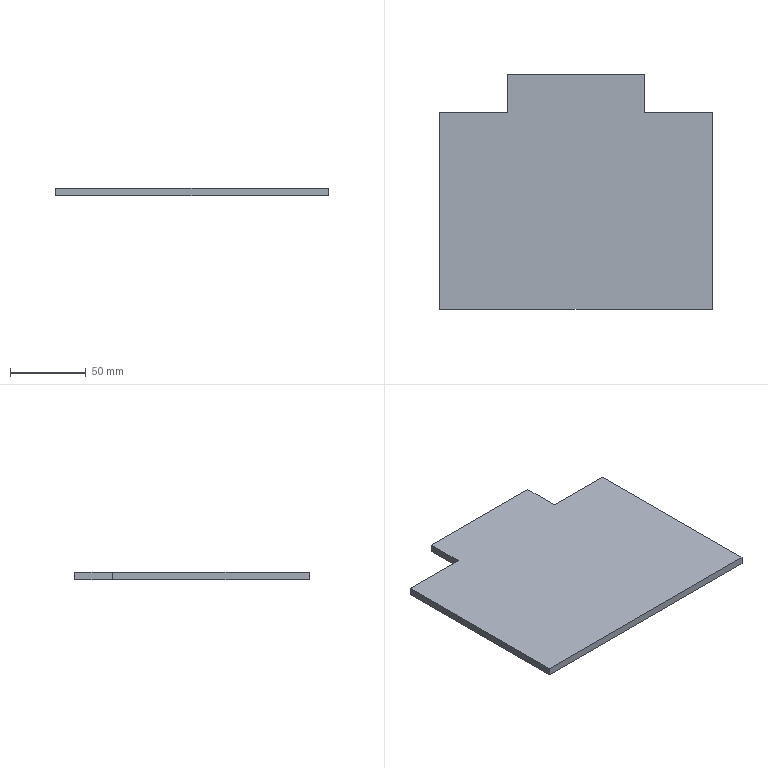Part | SolidWorks | features Extrusion 1, ICE 1 | 1 solid | 10 faces | box 180 x 155 x 5 mm | volume 128250 mm3 | plane 10
STEP:
#1=CARTESIAN_POINT('',(135.,0.,5.));
#2=VERTEX_POINT('',#1);
#3=CARTESIAN_POINT('',(135.,0.,0.));
#4=VERTEX_POINT('',#3);
#5=CARTESIAN_POINT('',(135.,0.,5.));
#6=DIRECTION('',(0.,0.,-1.));
#7=VECTOR('',#6,1000.);
#8=LINE('',#5,#7);
#9=EDGE_CURVE('',#2,#4,#8,.T.);
#10=ORIENTED_EDGE('',*,*,#9,.F.);
#11=CARTESIAN_POINT('',(180.,0.,5.));
#12=VERTEX_POINT('',#11);
#13=CARTESIAN_POINT('',(0.,0.,5.));
#14=DIRECTION('',(-1.,0.,0.));
#15=VECTOR('',#14,1000.);
#16=LINE('',#13,#15);
#17=EDGE_CURVE('',#12,#2,#16,.T.);
#18=ORIENTED_EDGE('',*,*,#17,.F.);
#19=CARTESIAN_POINT('',(180.,0.,0.));
#20=VERTEX_POINT('',#19);
#21=CARTESIAN_POINT('',(180.,0.,5.));
#22=DIRECTION('',(0.,0.,-1.));
#23=VECTOR('',#22,1000.);
#24=LINE('',#21,#23);
#25=EDGE_CURVE('',#12,#20,#24,.T.);
#26=ORIENTED_EDGE('',*,*,#25,.T.);
#27=CARTESIAN_POINT('',(0.,0.,0.));
#28=DIRECTION('',(-1.,0.,0.));
#29=VECTOR('',#28,1000.);
#30=LINE('',#27,#29);
#31=EDGE_CURVE('',#20,#4,#30,.T.);
#32=ORIENTED_EDGE('',*,*,#31,.T.);
#33=EDGE_LOOP('',(#10,#18,#26,#32));
#34=FACE_OUTER_BOUND('',#33,.T.);
#35=CARTESIAN_POINT('',(0.,0.,5.));
#36=DIRECTION('',(0.,-1.,0.));
#37=DIRECTION('',(0.,0.,-1.));
#38=AXIS2_PLACEMENT_3D('',#35,#36,#37);
#39=PLANE('',#38);
#40=ADVANCED_FACE('',(#34),#39,.F.);
#41=CARTESIAN_POINT('',(45.,0.,0.));
#42=VERTEX_POINT('',#41);
#43=CARTESIAN_POINT('',(45.,0.,5.));
#44=VERTEX_POINT('',#43);
#45=CARTESIAN_POINT('',(45.,0.,0.));
#46=DIRECTION('',(0.,0.,1.));
#47=VECTOR('',#46,1000.);
#48=LINE('',#45,#47);
#49=EDGE_CURVE('',#42,#44,#48,.T.);
#50=ORIENTED_EDGE('',*,*,#49,.F.);
#51=CARTESIAN_POINT('',(0.,0.,0.));
#52=VERTEX_POINT('',#51);
#53=CARTESIAN_POINT('',(0.,0.,0.));
#54=DIRECTION('',(-1.,0.,0.));
#55=VECTOR('',#54,1000.);
#56=LINE('',#53,#55);
#57=EDGE_CURVE('',#42,#52,#56,.T.);
#58=ORIENTED_EDGE('',*,*,#57,.T.);
#59=CARTESIAN_POINT('',(0.,0.,5.));
#60=VERTEX_POINT('',#59);
#61=CARTESIAN_POINT('',(0.,0.,5.));
#62=DIRECTION('',(0.,0.,-1.));
#63=VECTOR('',#62,1000.);
#64=LINE('',#61,#63);
#65=EDGE_CURVE('',#60,#52,#64,.T.);
#66=ORIENTED_EDGE('',*,*,#65,.F.);
#67=CARTESIAN_POINT('',(0.,0.,5.));
#68=DIRECTION('',(-1.,0.,0.));
#69=VECTOR('',#68,1000.);
#70=LINE('',#67,#69);
#71=EDGE_CURVE('',#44,#60,#70,.T.);
#72=ORIENTED_EDGE('',*,*,#71,.F.);
#73=EDGE_LOOP('',(#50,#58,#66,#72));
#74=FACE_OUTER_BOUND('',#73,.T.);
#75=CARTESIAN_POINT('',(0.,0.,5.));
#76=DIRECTION('',(0.,-1.,0.));
#77=DIRECTION('',(0.,0.,-1.));
#78=AXIS2_PLACEMENT_3D('',#75,#76,#77);
#79=PLANE('',#78);
#80=ADVANCED_FACE('',(#74),#79,.F.);
#81=CARTESIAN_POINT('',(0.,-130.,0.));
#82=VERTEX_POINT('',#81);
#83=CARTESIAN_POINT('',(0.,0.,0.));
#84=DIRECTION('',(0.,-1.,0.));
#85=VECTOR('',#84,1000.);
#86=LINE('',#83,#85);
#87=EDGE_CURVE('',#52,#82,#86,.T.);
#88=ORIENTED_EDGE('',*,*,#87,.T.);
#89=CARTESIAN_POINT('',(0.,-130.,5.));
#90=VERTEX_POINT('',#89);
#91=CARTESIAN_POINT('',(0.,-130.,5.));
#92=DIRECTION('',(0.,0.,-1.));
#93=VECTOR('',#92,1000.);
#94=LINE('',#91,#93);
#95=EDGE_CURVE('',#90,#82,#94,.T.);
#96=ORIENTED_EDGE('',*,*,#95,.F.);
#97=CARTESIAN_POINT('',(0.,0.,5.));
#98=DIRECTION('',(0.,-1.,0.));
#99=VECTOR('',#98,1000.);
#100=LINE('',#97,#99);
#101=EDGE_CURVE('',#60,#90,#100,.T.);
#102=ORIENTED_EDGE('',*,*,#101,.F.);
#103=ORIENTED_EDGE('',*,*,#65,.T.);
#104=EDGE_LOOP('',(#88,#96,#102,#103));
#105=FACE_OUTER_BOUND('',#104,.T.);
#106=CARTESIAN_POINT('',(0.,0.,5.));
#107=DIRECTION('',(1.,0.,0.));
#108=DIRECTION('',(0.,0.,-1.));
#109=AXIS2_PLACEMENT_3D('',#106,#107,#108);
#110=PLANE('',#109);
#111=ADVANCED_FACE('',(#105),#110,.F.);
#112=CARTESIAN_POINT('',(180.,-130.,0.));
#113=VERTEX_POINT('',#112);
#114=CARTESIAN_POINT('',(0.,-130.,0.));
#115=DIRECTION('',(1.,0.,0.));
#116=VECTOR('',#115,1000.);
#117=LINE('',#114,#116);
#118=EDGE_CURVE('',#82,#113,#117,.T.);
#119=ORIENTED_EDGE('',*,*,#118,.T.);
#120=CARTESIAN_POINT('',(180.,-130.,5.));
#121=VERTEX_POINT('',#120);
#122=CARTESIAN_POINT('',(180.,-130.,5.));
#123=DIRECTION('',(0.,0.,-1.));
#124=VECTOR('',#123,1000.);
#125=LINE('',#122,#124);
#126=EDGE_CURVE('',#121,#113,#125,.T.);
#127=ORIENTED_EDGE('',*,*,#126,.F.);
#128=CARTESIAN_POINT('',(0.,-130.,5.));
#129=DIRECTION('',(1.,0.,0.));
#130=VECTOR('',#129,1000.);
#131=LINE('',#128,#130);
#132=EDGE_CURVE('',#90,#121,#131,.T.);
#133=ORIENTED_EDGE('',*,*,#132,.F.);
#134=ORIENTED_EDGE('',*,*,#95,.T.);
#135=EDGE_LOOP('',(#119,#127,#133,#134));
#136=FACE_OUTER_BOUND('',#135,.T.);
#137=CARTESIAN_POINT('',(0.,-130.,5.));
#138=DIRECTION('',(0.,1.,0.));
#139=DIRECTION('',(0.,0.,1.));
#140=AXIS2_PLACEMENT_3D('',#137,#138,#139);
#141=PLANE('',#140);
#142=ADVANCED_FACE('',(#136),#141,.F.);
#143=CARTESIAN_POINT('',(180.,0.,0.));
#144=DIRECTION('',(0.,1.,0.));
#145=VECTOR('',#144,1000.);
#146=LINE('',#143,#145);
#147=EDGE_CURVE('',#113,#20,#146,.T.);
#148=ORIENTED_EDGE('',*,*,#147,.T.);
#149=ORIENTED_EDGE('',*,*,#25,.F.);
#150=CARTESIAN_POINT('',(180.,0.,5.));
#151=DIRECTION('',(0.,1.,0.));
#152=VECTOR('',#151,1000.);
#153=LINE('',#150,#152);
#154=EDGE_CURVE('',#121,#12,#153,.T.);
#155=ORIENTED_EDGE('',*,*,#154,.F.);
#156=ORIENTED_EDGE('',*,*,#126,.T.);
#157=EDGE_LOOP('',(#148,#149,#155,#156));
#158=FACE_OUTER_BOUND('',#157,.T.);
#159=CARTESIAN_POINT('',(180.,0.,5.));
#160=DIRECTION('',(-1.,0.,0.));
#161=DIRECTION('',(0.,-1.,0.));
#162=AXIS2_PLACEMENT_3D('',#159,#160,#161);
#163=PLANE('',#162);
#164=ADVANCED_FACE('',(#158),#163,.F.);
#165=ORIENTED_EDGE('',*,*,#101,.T.);
#166=ORIENTED_EDGE('',*,*,#132,.T.);
#167=ORIENTED_EDGE('',*,*,#154,.T.);
#168=ORIENTED_EDGE('',*,*,#17,.T.);
#169=CARTESIAN_POINT('',(135.,25.,5.));
#170=VERTEX_POINT('',#169);
#171=CARTESIAN_POINT('',(135.,25.,5.));
#172=DIRECTION('',(0.,-1.,0.));
#173=VECTOR('',#172,1000.);
#174=LINE('',#171,#173);
#175=EDGE_CURVE('',#170,#2,#174,.T.);
#176=ORIENTED_EDGE('',*,*,#175,.F.);
#177=CARTESIAN_POINT('',(45.,25.,5.));
#178=VERTEX_POINT('',#177);
#179=CARTESIAN_POINT('',(45.,25.,5.));
#180=DIRECTION('',(1.,0.,0.));
#181=VECTOR('',#180,1000.);
#182=LINE('',#179,#181);
#183=EDGE_CURVE('',#178,#170,#182,.T.);
#184=ORIENTED_EDGE('',*,*,#183,.F.);
#185=CARTESIAN_POINT('',(45.,25.,5.));
#186=DIRECTION('',(0.,-1.,0.));
#187=VECTOR('',#186,1000.);
#188=LINE('',#185,#187);
#189=EDGE_CURVE('',#178,#44,#188,.T.);
#190=ORIENTED_EDGE('',*,*,#189,.T.);
#191=ORIENTED_EDGE('',*,*,#71,.T.);
#192=EDGE_LOOP('',(#165,#166,#167,#168,#176,#184,#190,#191));
#193=FACE_OUTER_BOUND('',#192,.T.);
#194=CARTESIAN_POINT('',(0.,0.,5.));
#195=DIRECTION('',(0.,0.,1.));
#196=DIRECTION('',(1.,0.,0.));
#197=AXIS2_PLACEMENT_3D('',#194,#195,#196);
#198=PLANE('',#197);
#199=ADVANCED_FACE('',(#193),#198,.T.);
#200=ORIENTED_EDGE('',*,*,#87,.F.);
#201=ORIENTED_EDGE('',*,*,#57,.F.);
#202=CARTESIAN_POINT('',(45.,25.,0.));
#203=VERTEX_POINT('',#202);
#204=CARTESIAN_POINT('',(45.,25.,0.));
#205=DIRECTION('',(0.,-1.,0.));
#206=VECTOR('',#205,1000.);
#207=LINE('',#204,#206);
#208=EDGE_CURVE('',#203,#42,#207,.T.);
#209=ORIENTED_EDGE('',*,*,#208,.F.);
#210=CARTESIAN_POINT('',(135.,25.,0.));
#211=VERTEX_POINT('',#210);
#212=CARTESIAN_POINT('',(45.,25.,0.));
#213=DIRECTION('',(-1.,0.,0.));
#214=VECTOR('',#213,1000.);
#215=LINE('',#212,#214);
#216=EDGE_CURVE('',#211,#203,#215,.T.);
#217=ORIENTED_EDGE('',*,*,#216,.F.);
#218=CARTESIAN_POINT('',(135.,25.,0.));
#219=DIRECTION('',(0.,-1.,0.));
#220=VECTOR('',#219,1000.);
#221=LINE('',#218,#220);
#222=EDGE_CURVE('',#211,#4,#221,.T.);
#223=ORIENTED_EDGE('',*,*,#222,.T.);
#224=ORIENTED_EDGE('',*,*,#31,.F.);
#225=ORIENTED_EDGE('',*,*,#147,.F.);
#226=ORIENTED_EDGE('',*,*,#118,.F.);
#227=EDGE_LOOP('',(#200,#201,#209,#217,#223,#224,#225,#226));
#228=FACE_OUTER_BOUND('',#227,.T.);
#229=CARTESIAN_POINT('',(0.,0.,0.));
#230=DIRECTION('',(0.,0.,1.));
#231=DIRECTION('',(1.,0.,0.));
#232=AXIS2_PLACEMENT_3D('',#229,#230,#231);
#233=PLANE('',#232);
#234=ADVANCED_FACE('',(#228),#233,.F.);
#235=ORIENTED_EDGE('',*,*,#9,.T.);
#236=ORIENTED_EDGE('',*,*,#222,.F.);
#237=CARTESIAN_POINT('',(135.,25.,5.));
#238=DIRECTION('',(0.,0.,-1.));
#239=VECTOR('',#238,1000.);
#240=LINE('',#237,#239);
#241=EDGE_CURVE('',#170,#211,#240,.T.);
#242=ORIENTED_EDGE('',*,*,#241,.F.);
#243=ORIENTED_EDGE('',*,*,#175,.T.);
#244=EDGE_LOOP('',(#235,#236,#242,#243));
#245=FACE_OUTER_BOUND('',#244,.T.);
#246=CARTESIAN_POINT('',(135.,25.,5.));
#247=DIRECTION('',(-1.,0.,0.));
#248=DIRECTION('',(0.,0.,1.));
#249=AXIS2_PLACEMENT_3D('',#246,#247,#248);
#250=PLANE('',#249);
#251=ADVANCED_FACE('',(#245),#250,.F.);
#252=ORIENTED_EDGE('',*,*,#49,.T.);
#253=ORIENTED_EDGE('',*,*,#189,.F.);
#254=CARTESIAN_POINT('',(45.,25.,0.));
#255=DIRECTION('',(0.,0.,1.));
#256=VECTOR('',#255,1000.);
#257=LINE('',#254,#256);
#258=EDGE_CURVE('',#203,#178,#257,.T.);
#259=ORIENTED_EDGE('',*,*,#258,.F.);
#260=ORIENTED_EDGE('',*,*,#208,.T.);
#261=EDGE_LOOP('',(#252,#253,#259,#260));
#262=FACE_OUTER_BOUND('',#261,.T.);
#263=CARTESIAN_POINT('',(45.,25.,0.));
#264=DIRECTION('',(1.,0.,0.));
#265=DIRECTION('',(0.,0.,-1.));
#266=AXIS2_PLACEMENT_3D('',#263,#264,#265);
#267=PLANE('',#266);
#268=ADVANCED_FACE('',(#262),#267,.F.);
#269=ORIENTED_EDGE('',*,*,#241,.T.);
#270=ORIENTED_EDGE('',*,*,#216,.T.);
#271=ORIENTED_EDGE('',*,*,#258,.T.);
#272=ORIENTED_EDGE('',*,*,#183,.T.);
#273=EDGE_LOOP('',(#269,#270,#271,#272));
#274=FACE_OUTER_BOUND('',#273,.T.);
#275=CARTESIAN_POINT('',(0.,25.,0.));
#276=DIRECTION('',(0.,-1.,0.));
#277=DIRECTION('',(0.,0.,-1.));
#278=AXIS2_PLACEMENT_3D('',#275,#276,#277);
#279=PLANE('',#278);
#280=ADVANCED_FACE('',(#274),#279,.F.);
#281=CLOSED_SHELL('',(#40,#80,#111,#142,#164,#199,#234,#251,#268,#280));
#282=MANIFOLD_SOLID_BREP('',#281);
#283=CARTESIAN_POINT('',(0.,0.,0.));
#284=DIRECTION('',(0.,0.,1.));
#285=DIRECTION('',(1.,0.,0.));
#286=AXIS2_PLACEMENT_3D('',#283,#284,#285);
#287=(LENGTH_UNIT()NAMED_UNIT(*)SI_UNIT(.MILLI.,.METRE.));
#288=UNCERTAINTY_MEASURE_WITH_UNIT(LENGTH_MEASURE(0.00001),#287,'','');
#289=(NAMED_UNIT(*)PLANE_ANGLE_UNIT()SI_UNIT($,.RADIAN.));
#290=(NAMED_UNIT(*)SI_UNIT($,.STERADIAN.)SOLID_ANGLE_UNIT());
#291=(GEOMETRIC_REPRESENTATION_CONTEXT(3)GLOBAL_UNCERTAINTY_ASSIGNED_CONTEXT((#288))GLOBAL_UNIT_ASSIGNED_CONTEXT((#287,#289,#290))REPRESENTATION_CONTEXT('',''));
#292=ADVANCED_BREP_SHAPE_REPRESENTATION('',(#282,#286),#291);